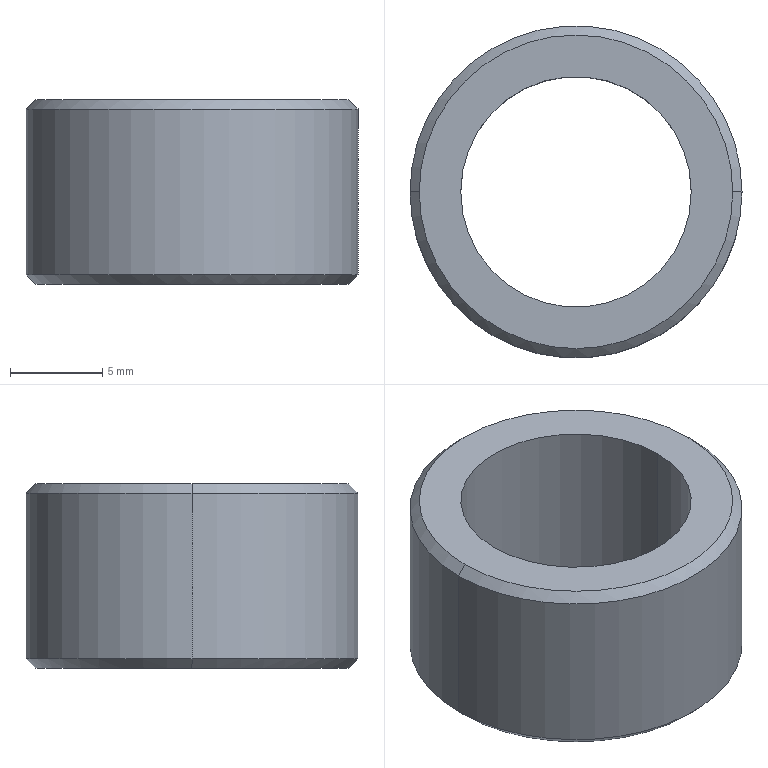Part | SolidWorks | features Chamfer 1, Extrusion 1 | 1 solid | 10 faces | box 18 x 18 x 10 mm | volume 1304 mm3 | cone 4 | cylinder 4 | plane 2 | commonest cylinder face diameters 12.5 x2 18 x2
STEP:
#1=CARTESIAN_POINT('',(-8.5,0.,0.));
#2=VERTEX_POINT('',#1);
#3=CARTESIAN_POINT('',(8.5,0.,0.));
#4=VERTEX_POINT('',#3);
#5=CARTESIAN_POINT('',(0.,0.,0.));
#6=DIRECTION('',(0.,0.,-1.));
#7=DIRECTION('',(1.,0.,0.));
#8=AXIS2_PLACEMENT_3D('',#5,#6,#7);
#9=CIRCLE('',#8,8.5);
#10=EDGE_CURVE('',#2,#4,#9,.T.);
#11=ORIENTED_EDGE('',*,*,#10,.F.);
#12=CARTESIAN_POINT('',(-9.,0.,0.5));
#13=VERTEX_POINT('',#12);
#14=CARTESIAN_POINT('',(-9.,0.,0.5));
#15=DIRECTION('',(-0.7071,0.,0.7071));
#16=VECTOR('',#15,1000.);
#17=LINE('',#14,#16);
#18=EDGE_CURVE('',#2,#13,#17,.T.);
#19=ORIENTED_EDGE('',*,*,#18,.T.);
#20=CARTESIAN_POINT('',(9.,0.,0.5));
#21=VERTEX_POINT('',#20);
#22=CARTESIAN_POINT('',(0.,0.,0.5));
#23=DIRECTION('',(0.,0.,1.));
#24=DIRECTION('',(1.,0.,0.));
#25=AXIS2_PLACEMENT_3D('',#22,#23,#24);
#26=CIRCLE('',#25,9.);
#27=EDGE_CURVE('',#21,#13,#26,.T.);
#28=ORIENTED_EDGE('',*,*,#27,.F.);
#29=CARTESIAN_POINT('',(9.,0.,0.5));
#30=DIRECTION('',(0.7071,0.,0.7071));
#31=VECTOR('',#30,1000.);
#32=LINE('',#29,#31);
#33=EDGE_CURVE('',#4,#21,#32,.T.);
#34=ORIENTED_EDGE('',*,*,#33,.F.);
#35=EDGE_LOOP('',(#11,#19,#28,#34));
#36=FACE_OUTER_BOUND('',#35,.T.);
#37=CARTESIAN_POINT('',(0.,0.,0.5));
#38=DIRECTION('',(0.,0.,1.));
#39=DIRECTION('',(1.,0.,0.));
#40=AXIS2_PLACEMENT_3D('',#37,#38,#39);
#41=CONICAL_SURFACE('',#40,9.,0.7854);
#42=ADVANCED_FACE('',(#36),#41,.T.);
#43=CARTESIAN_POINT('',(8.5,0.,10.));
#44=VERTEX_POINT('',#43);
#45=CARTESIAN_POINT('',(-8.5,0.,10.));
#46=VERTEX_POINT('',#45);
#47=CARTESIAN_POINT('',(0.,0.,10.));
#48=DIRECTION('',(0.,0.,1.));
#49=DIRECTION('',(1.,0.,0.));
#50=AXIS2_PLACEMENT_3D('',#47,#48,#49);
#51=CIRCLE('',#50,8.5);
#52=EDGE_CURVE('',#44,#46,#51,.T.);
#53=ORIENTED_EDGE('',*,*,#52,.F.);
#54=CARTESIAN_POINT('',(9.,0.,9.5));
#55=VERTEX_POINT('',#54);
#56=CARTESIAN_POINT('',(8.5,0.,10.));
#57=DIRECTION('',(0.7071,0.,-0.7071));
#58=VECTOR('',#57,1000.);
#59=LINE('',#56,#58);
#60=EDGE_CURVE('',#44,#55,#59,.T.);
#61=ORIENTED_EDGE('',*,*,#60,.T.);
#62=CARTESIAN_POINT('',(-9.,0.,9.5));
#63=VERTEX_POINT('',#62);
#64=CARTESIAN_POINT('',(0.,0.,9.5));
#65=DIRECTION('',(0.,0.,-1.));
#66=DIRECTION('',(1.,0.,0.));
#67=AXIS2_PLACEMENT_3D('',#64,#65,#66);
#68=CIRCLE('',#67,9.);
#69=EDGE_CURVE('',#63,#55,#68,.T.);
#70=ORIENTED_EDGE('',*,*,#69,.F.);
#71=CARTESIAN_POINT('',(-8.5,0.,10.));
#72=DIRECTION('',(-0.7071,0.,-0.7071));
#73=VECTOR('',#72,1000.);
#74=LINE('',#71,#73);
#75=EDGE_CURVE('',#46,#63,#74,.T.);
#76=ORIENTED_EDGE('',*,*,#75,.F.);
#77=EDGE_LOOP('',(#53,#61,#70,#76));
#78=FACE_OUTER_BOUND('',#77,.T.);
#79=CARTESIAN_POINT('',(0.,0.,10.));
#80=DIRECTION('',(0.,0.,-1.));
#81=DIRECTION('',(-1.,0.,0.));
#82=AXIS2_PLACEMENT_3D('',#79,#80,#81);
#83=CONICAL_SURFACE('',#82,8.5,0.7854);
#84=ADVANCED_FACE('',(#78),#83,.T.);
#85=CARTESIAN_POINT('',(-6.25,0.,10.));
#86=VERTEX_POINT('',#85);
#87=CARTESIAN_POINT('',(6.25,0.,10.));
#88=VERTEX_POINT('',#87);
#89=CARTESIAN_POINT('',(0.,0.,10.));
#90=DIRECTION('',(0.,0.,1.));
#91=DIRECTION('',(1.,0.,0.));
#92=AXIS2_PLACEMENT_3D('',#89,#90,#91);
#93=CIRCLE('',#92,6.25);
#94=EDGE_CURVE('',#86,#88,#93,.T.);
#95=ORIENTED_EDGE('',*,*,#94,.T.);
#96=CARTESIAN_POINT('',(6.25,0.,0.));
#97=VERTEX_POINT('',#96);
#98=CARTESIAN_POINT('',(6.25,0.,10.));
#99=DIRECTION('',(0.,0.,-1.));
#100=VECTOR('',#99,1000.);
#101=LINE('',#98,#100);
#102=EDGE_CURVE('',#88,#97,#101,.T.);
#103=ORIENTED_EDGE('',*,*,#102,.T.);
#104=CARTESIAN_POINT('',(-6.25,0.,0.));
#105=VERTEX_POINT('',#104);
#106=CARTESIAN_POINT('',(0.,0.,0.));
#107=DIRECTION('',(0.,0.,1.));
#108=DIRECTION('',(1.,0.,0.));
#109=AXIS2_PLACEMENT_3D('',#106,#107,#108);
#110=CIRCLE('',#109,6.25);
#111=EDGE_CURVE('',#105,#97,#110,.T.);
#112=ORIENTED_EDGE('',*,*,#111,.F.);
#113=CARTESIAN_POINT('',(-6.25,0.,10.));
#114=DIRECTION('',(0.,0.,-1.));
#115=VECTOR('',#114,1000.);
#116=LINE('',#113,#115);
#117=EDGE_CURVE('',#86,#105,#116,.T.);
#118=ORIENTED_EDGE('',*,*,#117,.F.);
#119=EDGE_LOOP('',(#95,#103,#112,#118));
#120=FACE_OUTER_BOUND('',#119,.T.);
#121=CARTESIAN_POINT('',(0.,0.,10.));
#122=DIRECTION('',(0.,0.,-1.));
#123=DIRECTION('',(-1.,0.,0.));
#124=AXIS2_PLACEMENT_3D('',#121,#122,#123);
#125=CYLINDRICAL_SURFACE('',#124,6.25);
#126=ADVANCED_FACE('',(#120),#125,.F.);
#127=ORIENTED_EDGE('',*,*,#69,.T.);
#128=CARTESIAN_POINT('',(9.,0.,10.));
#129=DIRECTION('',(0.,0.,-1.));
#130=VECTOR('',#129,1000.);
#131=LINE('',#128,#130);
#132=EDGE_CURVE('',#55,#21,#131,.T.);
#133=ORIENTED_EDGE('',*,*,#132,.T.);
#134=ORIENTED_EDGE('',*,*,#27,.T.);
#135=CARTESIAN_POINT('',(-9.,0.,10.));
#136=DIRECTION('',(0.,0.,-1.));
#137=VECTOR('',#136,1000.);
#138=LINE('',#135,#137);
#139=EDGE_CURVE('',#63,#13,#138,.T.);
#140=ORIENTED_EDGE('',*,*,#139,.F.);
#141=EDGE_LOOP('',(#127,#133,#134,#140));
#142=FACE_OUTER_BOUND('',#141,.T.);
#143=CARTESIAN_POINT('',(0.,0.,10.));
#144=DIRECTION('',(0.,0.,-1.));
#145=DIRECTION('',(-1.,0.,0.));
#146=AXIS2_PLACEMENT_3D('',#143,#144,#145);
#147=CYLINDRICAL_SURFACE('',#146,9.);
#148=ADVANCED_FACE('',(#142),#147,.T.);
#149=CARTESIAN_POINT('',(0.,0.,10.));
#150=DIRECTION('',(0.,0.,1.));
#151=DIRECTION('',(1.,0.,0.));
#152=AXIS2_PLACEMENT_3D('',#149,#150,#151);
#153=CIRCLE('',#152,8.5);
#154=EDGE_CURVE('',#46,#44,#153,.T.);
#155=ORIENTED_EDGE('',*,*,#154,.T.);
#156=ORIENTED_EDGE('',*,*,#52,.T.);
#157=EDGE_LOOP('',(#155,#156));
#158=FACE_OUTER_BOUND('',#157,.T.);
#159=ORIENTED_EDGE('',*,*,#94,.F.);
#160=CARTESIAN_POINT('',(0.,0.,10.));
#161=DIRECTION('',(0.,0.,1.));
#162=DIRECTION('',(1.,0.,0.));
#163=AXIS2_PLACEMENT_3D('',#160,#161,#162);
#164=CIRCLE('',#163,6.25);
#165=EDGE_CURVE('',#88,#86,#164,.T.);
#166=ORIENTED_EDGE('',*,*,#165,.F.);
#167=EDGE_LOOP('',(#159,#166));
#168=FACE_BOUND('',#167,.T.);
#169=CARTESIAN_POINT('',(0.,0.,10.));
#170=DIRECTION('',(0.,0.,1.));
#171=DIRECTION('',(1.,0.,0.));
#172=AXIS2_PLACEMENT_3D('',#169,#170,#171);
#173=PLANE('',#172);
#174=ADVANCED_FACE('',(#158,#168),#173,.T.);
#175=CARTESIAN_POINT('',(0.,0.,0.));
#176=DIRECTION('',(0.,0.,-1.));
#177=DIRECTION('',(1.,0.,0.));
#178=AXIS2_PLACEMENT_3D('',#175,#176,#177);
#179=CIRCLE('',#178,8.5);
#180=EDGE_CURVE('',#4,#2,#179,.T.);
#181=ORIENTED_EDGE('',*,*,#180,.T.);
#182=ORIENTED_EDGE('',*,*,#10,.T.);
#183=EDGE_LOOP('',(#181,#182));
#184=FACE_OUTER_BOUND('',#183,.T.);
#185=ORIENTED_EDGE('',*,*,#111,.T.);
#186=CARTESIAN_POINT('',(0.,0.,0.));
#187=DIRECTION('',(0.,0.,1.));
#188=DIRECTION('',(1.,0.,0.));
#189=AXIS2_PLACEMENT_3D('',#186,#187,#188);
#190=CIRCLE('',#189,6.25);
#191=EDGE_CURVE('',#97,#105,#190,.T.);
#192=ORIENTED_EDGE('',*,*,#191,.T.);
#193=EDGE_LOOP('',(#185,#192));
#194=FACE_BOUND('',#193,.T.);
#195=CARTESIAN_POINT('',(0.,0.,0.));
#196=DIRECTION('',(0.,0.,1.));
#197=DIRECTION('',(1.,0.,0.));
#198=AXIS2_PLACEMENT_3D('',#195,#196,#197);
#199=PLANE('',#198);
#200=ADVANCED_FACE('',(#184,#194),#199,.F.);
#201=ORIENTED_EDGE('',*,*,#132,.F.);
#202=CARTESIAN_POINT('',(0.,0.,9.5));
#203=DIRECTION('',(0.,0.,-1.));
#204=DIRECTION('',(1.,0.,0.));
#205=AXIS2_PLACEMENT_3D('',#202,#203,#204);
#206=CIRCLE('',#205,9.);
#207=EDGE_CURVE('',#55,#63,#206,.T.);
#208=ORIENTED_EDGE('',*,*,#207,.T.);
#209=ORIENTED_EDGE('',*,*,#139,.T.);
#210=CARTESIAN_POINT('',(0.,0.,0.5));
#211=DIRECTION('',(0.,0.,1.));
#212=DIRECTION('',(1.,0.,0.));
#213=AXIS2_PLACEMENT_3D('',#210,#211,#212);
#214=CIRCLE('',#213,9.);
#215=EDGE_CURVE('',#13,#21,#214,.T.);
#216=ORIENTED_EDGE('',*,*,#215,.T.);
#217=EDGE_LOOP('',(#201,#208,#209,#216));
#218=FACE_OUTER_BOUND('',#217,.T.);
#219=CARTESIAN_POINT('',(0.,0.,10.));
#220=DIRECTION('',(0.,0.,-1.));
#221=DIRECTION('',(-1.,0.,0.));
#222=AXIS2_PLACEMENT_3D('',#219,#220,#221);
#223=CYLINDRICAL_SURFACE('',#222,9.);
#224=ADVANCED_FACE('',(#218),#223,.T.);
#225=ORIENTED_EDGE('',*,*,#102,.F.);
#226=ORIENTED_EDGE('',*,*,#165,.T.);
#227=ORIENTED_EDGE('',*,*,#117,.T.);
#228=ORIENTED_EDGE('',*,*,#191,.F.);
#229=EDGE_LOOP('',(#225,#226,#227,#228));
#230=FACE_OUTER_BOUND('',#229,.T.);
#231=CARTESIAN_POINT('',(0.,0.,10.));
#232=DIRECTION('',(0.,0.,-1.));
#233=DIRECTION('',(-1.,0.,0.));
#234=AXIS2_PLACEMENT_3D('',#231,#232,#233);
#235=CYLINDRICAL_SURFACE('',#234,6.25);
#236=ADVANCED_FACE('',(#230),#235,.F.);
#237=ORIENTED_EDGE('',*,*,#60,.F.);
#238=ORIENTED_EDGE('',*,*,#154,.F.);
#239=ORIENTED_EDGE('',*,*,#75,.T.);
#240=ORIENTED_EDGE('',*,*,#207,.F.);
#241=EDGE_LOOP('',(#237,#238,#239,#240));
#242=FACE_OUTER_BOUND('',#241,.T.);
#243=CARTESIAN_POINT('',(0.,0.,10.));
#244=DIRECTION('',(0.,0.,-1.));
#245=DIRECTION('',(-1.,0.,0.));
#246=AXIS2_PLACEMENT_3D('',#243,#244,#245);
#247=CONICAL_SURFACE('',#246,8.5,0.7854);
#248=ADVANCED_FACE('',(#242),#247,.T.);
#249=ORIENTED_EDGE('',*,*,#18,.F.);
#250=ORIENTED_EDGE('',*,*,#180,.F.);
#251=ORIENTED_EDGE('',*,*,#33,.T.);
#252=ORIENTED_EDGE('',*,*,#215,.F.);
#253=EDGE_LOOP('',(#249,#250,#251,#252));
#254=FACE_OUTER_BOUND('',#253,.T.);
#255=CARTESIAN_POINT('',(0.,0.,0.5));
#256=DIRECTION('',(0.,0.,1.));
#257=DIRECTION('',(1.,0.,0.));
#258=AXIS2_PLACEMENT_3D('',#255,#256,#257);
#259=CONICAL_SURFACE('',#258,9.,0.7854);
#260=ADVANCED_FACE('',(#254),#259,.T.);
#261=CLOSED_SHELL('',(#42,#84,#126,#148,#174,#200,#224,#236,#248,#260));
#262=MANIFOLD_SOLID_BREP('',#261);
#263=CARTESIAN_POINT('',(0.,0.,0.));
#264=DIRECTION('',(0.,0.,1.));
#265=DIRECTION('',(1.,0.,0.));
#266=AXIS2_PLACEMENT_3D('',#263,#264,#265);
#267=(LENGTH_UNIT()NAMED_UNIT(*)SI_UNIT(.MILLI.,.METRE.));
#268=UNCERTAINTY_MEASURE_WITH_UNIT(LENGTH_MEASURE(0.00001),#267,'','');
#269=(NAMED_UNIT(*)PLANE_ANGLE_UNIT()SI_UNIT($,.RADIAN.));
#270=(NAMED_UNIT(*)SI_UNIT($,.STERADIAN.)SOLID_ANGLE_UNIT());
#271=(GEOMETRIC_REPRESENTATION_CONTEXT(3)GLOBAL_UNCERTAINTY_ASSIGNED_CONTEXT((#268))GLOBAL_UNIT_ASSIGNED_CONTEXT((#267,#269,#270))REPRESENTATION_CONTEXT('',''));
#272=ADVANCED_BREP_SHAPE_REPRESENTATION('',(#262,#266),#271);